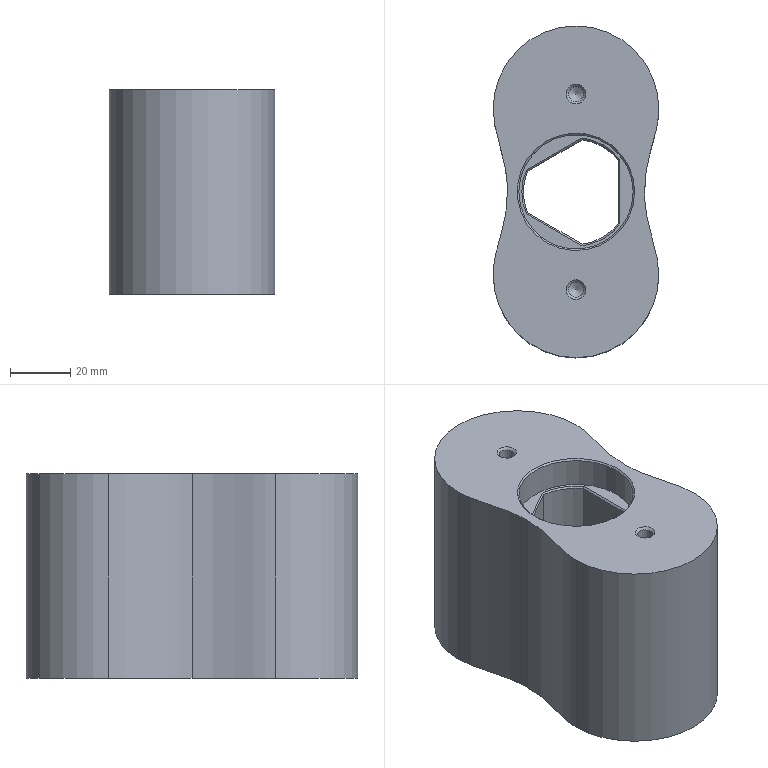NC program | NX | posted with a generic post | part box 55.004 x 110.159 x 68 mm
Lines 15415 to 16245 of 17802:
(CUTTERCOMP12 , TOOL : D12)
N30822 T12 M6
N30824 G54
N30826 G17 G0 G90 X-29.641 Y35.939 S5000 M3
N30828 G43 Z30. H12
N30830 Z1.
N30832 G94 G1 Z-1. F1250.
N30834 G41 X-29.607 Y35.845 D12
N30836 X-28.613 Y34.106
N30838 G3 X-27.576 Y33.502 R1.2
N30840 G2 X-20.525 Y32.77 R35.7
N30842 X-16.127 Y31.691 R60.387
N30844 G1 X-12.217 Y30.6
N30846 X-11.729 Y30.47
N30848 G3 X-6.353 Y29.294 R55.332
N30850 X6.353 Y29.294 R38.755
N30852 X11.729 Y30.47 R55.4
N30854 X16.345 Y31.754 R390.707
N30856 G2 X20.525 Y32.77 R61.951
N30858 X27.576 Y33.502 R35.718
N30860 X61.079 Y0.001 R33.502
N30862 X27.576 Y-33.502 R33.502
N30864 X20.525 Y-32.77 R35.7
N30866 X16.127 Y-31.691 R60.389
N30868 G1 X12.217 Y-30.6
N30870 X11.729 Y-30.47
N30872 G3 X6.353 Y-29.295 R55.338
N30874 X-6.353 Y-29.295 R38.754
N30876 X-11.729 Y-30.47 R55.381
N30878 X-16.345 Y-31.754 R390.608
N30880 G2 X-20.525 Y-32.77 R61.945
N30882 X-27.576 Y-33.502 R35.716
N30884 X-61.079 Y-0.001 R33.502
N30886 X-27.576 Y33.502 R33.502
N30888 G3 X-26.537 Y34.102 R1.2
N30890 G1 X-25.534 Y35.84
N30892 G40
N30894 X-25.5 Y35.934
N30896 Z1.
N30898 G0 X-29.641 Y35.939 Z0.
N30900 G1 Z-2.
N30902 G41 X-29.607 Y35.845
N30904 X-28.613 Y34.106
N30906 G3 X-27.576 Y33.502 R1.2
N30908 G2 X-20.525 Y32.77 R35.7
N30910 X-16.127 Y31.691 R60.387
N30912 G1 X-12.217 Y30.6
N30914 X-11.729 Y30.47
N30916 G3 X-6.353 Y29.295 R55.33
N30918 X6.353 Y29.295 R38.754
N30920 X11.729 Y30.47 R55.601
N30922 X16.345 Y31.754 R390.532
N30924 G2 X20.525 Y32.77 R61.937
N30926 X27.576 Y33.502 R35.715
N30928 X61.079 Y0.001 R33.502
N30930 X27.576 Y-33.502 R33.502
N30932 X20.036 Y-32.668 R36.091
N30934 X15.638 Y-31.556 R68.692
N30936 G3 X11.24 Y-30.342 R232.507
N30938 X5.864 Y-29.216 R53.118
N30940 X-6.353 Y-29.295 R38.762
N30942 X-11.729 Y-30.47 R55.563
N30944 X-16.345 Y-31.754 R390.333
N30946 G2 X-20.525 Y-32.77 R61.924
N30948 X-27.576 Y-33.502 R35.711
N30950 X-61.079 Y-0.001 R33.502
N30952 X-27.576 Y33.502 R33.502
N30954 G3 X-26.537 Y34.102 R1.2
N30956 G1 X-25.534 Y35.84
N30958 G40
N30960 X-25.5 Y35.934
N30962 Z0.
N30964 G0 X-29.641 Y35.939 Z-1.
N30966 G1 Z-3.
N30968 G41 X-29.607 Y35.845
N30970 X-28.613 Y34.106
N30972 G3 X-27.576 Y33.502 R1.2
N30974 G2 X-20.525 Y32.77 R35.7
N30976 X-16.127 Y31.691 R60.387
N30978 G1 X-12.217 Y30.6
N30980 X-11.729 Y30.47
N30982 G3 X-6.353 Y29.295 R55.328
N30984 X6.353 Y29.295 R38.753
N30986 X11.729 Y30.47 R55.578
N30988 X16.345 Y31.754 R390.357
N30990 G2 X20.525 Y32.77 R61.923
N30992 X27.576 Y33.502 R35.712
N30994 X61.079 Y0.001 R33.502
N30996 X27.576 Y-33.502 R33.502
N30998 X20.036 Y-32.669 R36.088
N31000 X15.638 Y-31.556 R68.743
N31002 G3 X11.24 Y-30.342 R232.194
N31004 X5.864 Y-29.216 R53.103
N31006 X-6.353 Y-29.295 R38.76
N31008 X-11.729 Y-30.47 R55.521
N31010 X-16.345 Y-31.754 R390.059
N31012 G2 X-20.525 Y-32.77 R61.903
N31014 X-27.576 Y-33.502 R35.706
N31016 X-61.079 Y-0.001 R33.502
N31018 X-27.576 Y33.502 R33.502
N31020 G3 X-26.537 Y34.102 R1.2
N31022 G1 X-25.534 Y35.84
N31024 G40
N31026 X-25.5 Y35.934
N31028 Z-1.
N31030 G0 X-29.641 Y35.939 Z-2.
N31032 G1 Z-4.
N31034 G41 X-29.607 Y35.845
N31036 X-28.613 Y34.106
N31038 G3 X-27.576 Y33.502 R1.2
N31040 G2 X-20.525 Y32.77 R35.7
N31042 X-16.127 Y31.691 R60.387
N31044 G1 X-12.217 Y30.6
N31046 X-11.729 Y30.47
N31048 G3 X-6.353 Y29.295 R55.326
N31050 X6.353 Y29.295 R38.752
N31052 X11.729 Y30.47 R55.555
N31054 X16.345 Y31.754 R390.181
N31056 G2 X20.525 Y32.77 R61.909
N31058 X27.576 Y33.502 R35.709
N31060 X61.079 Y0.001 R33.502
N31062 X27.576 Y-33.502 R33.502
N31064 X20.036 Y-32.669 R36.084
N31066 X15.638 Y-31.556 R68.794
N31068 G3 X11.24 Y-30.342 R231.881
N31070 X5.864 Y-29.216 R53.066
N31072 X-6.353 Y-29.295 R38.758
N31074 X-11.729 Y-30.47 R55.48
N31076 X-16.345 Y-31.754 R389.785
N31078 G2 X-20.525 Y-32.77 R61.882
N31080 X-27.576 Y-33.502 R35.629
N31082 X-61.079 Y-0.001 R33.502
N31084 X-27.576 Y33.502 R33.502
N31086 G3 X-26.537 Y34.102 R1.2
N31088 G1 X-25.534 Y35.84
N31090 G40
N31092 X-25.5 Y35.934
N31094 Z-2.
N31096 G0 X-29.638 Y35.939 Z-3.
N31098 G1 Z-5.
N31100 G41 X-29.605 Y35.845
N31102 X-28.612 Y34.107
N31104 G3 X-27.576 Y33.502 R1.2
N31106 G2 X-20.036 Y32.669 R36.084
N31108 X-15.638 Y31.556 R68.651
N31110 G3 X-11.24 Y30.342 R232.92
N31112 X-5.864 Y29.216 R53.116
N31114 X6.353 Y29.295 R38.761
N31116 X11.729 Y30.47 R55.532
N31118 X16.345 Y31.754 R390.007
N31120 G2 X20.525 Y32.77 R61.894
N31122 X27.576 Y33.502 R35.706
N31124 X61.079 Y0.001 R33.502
N31126 X27.576 Y-33.502 R33.502
N31128 X20.036 Y-32.669 R36.081
N31130 X15.638 Y-31.556 R68.83
N31132 G3 X11.24 Y-30.342 R231.57
N31134 X5.864 Y-29.217 R53.057
N31136 X-6.353 Y-29.295 R38.755
N31138 X-11.729 Y-30.47 R55.465
N31140 X-16.344 Y-31.754 R389.512
N31142 G2 X-20.525 Y-32.77 R61.861
N31144 X-27.576 Y-33.502 R35.624
N31146 X-61.079 Y-0.001 R33.502
N31148 X-27.576 Y33.502 R33.502
N31150 G3 X-26.537 Y34.102 R1.2
N31152 G1 X-25.534 Y35.839
N31154 G40
N31156 X-25.5 Y35.933
N31158 Z-3.
N31160 G0 X-29.641 Y35.939 Z-4.
N31162 G1 Z-6.
N31164 G41 X-29.607 Y35.845
N31166 X-28.613 Y34.106
N31168 G3 X-27.576 Y33.502 R1.2
N31170 G2 X-20.525 Y32.77 R35.701
N31172 X-16.127 Y31.691 R60.387
N31174 G1 X-12.217 Y30.6
N31176 X-11.729 Y30.47
N31178 G3 X-6.289 Y29.285 R54.809
N31180 X6.405 Y29.303 R38.597
N31182 X11.729 Y30.47 R55.51
N31184 X16.345 Y31.754 R389.832
N31186 G2 X20.525 Y32.77 R61.88
N31188 X27.576 Y33.502 R35.632
N31190 X61.079 Y0.001 R33.502
N31192 X27.576 Y-33.502 R33.502
N31194 X20.036 Y-32.669 R36.078
N31196 X15.638 Y-31.556 R68.857
N31198 G3 X11.24 Y-30.342 R231.258
N31200 X5.864 Y-29.217 R53.048
N31202 X-6.353 Y-29.295 R38.753
N31204 X-11.729 Y-30.47 R55.459
N31206 X-16.344 Y-31.754 R389.238
N31208 G2 X-20.525 Y-32.77 R61.84
N31210 X-27.576 Y-33.502 R35.619
N31212 X-61.079 Y-0.001 R33.502
N31214 X-27.576 Y33.502 R33.502
N31216 G3 X-26.537 Y34.102 R1.2
N31218 G1 X-25.534 Y35.84
N31220 G40
N31222 X-25.5 Y35.934
N31224 Z-4.
N31226 G0 X-29.641 Y35.939 Z-5.
N31228 G1 Z-7.
N31230 G41 X-29.607 Y35.845
N31232 X-28.613 Y34.106
N31234 G3 X-27.576 Y33.502 R1.2
N31236 G2 X-20.525 Y32.77 R35.7
N31238 X-16.127 Y31.691 R60.387
N31240 G1 X-12.217 Y30.6
N31242 X-11.729 Y30.47
N31244 G3 X-6.287 Y29.284 R54.784
N31246 X6.402 Y29.303 R38.597
N31248 X11.729 Y30.47 R55.487
N31250 X16.345 Y31.754 R389.657
N31252 G2 X20.525 Y32.77 R61.866
N31254 X27.576 Y33.502 R35.629
N31256 X61.079 Y0.001 R33.502
N31258 X27.576 Y-33.502 R33.502
N31260 X20.036 Y-32.669 R36.074
N31262 X15.638 Y-31.556 R68.884
N31264 G3 X11.24 Y-30.342 R233.491
N31266 X5.864 Y-29.217 R53.039
N31268 X-6.353 Y-29.295 R38.751
N31270 X-11.729 Y-30.47 R55.356
N31272 X-16.344 Y-31.754 R388.965
N31274 G2 X-20.525 Y-32.77 R61.819
N31276 X-27.576 Y-33.502 R35.613
N31278 X-61.079 Y-0.001 R33.502
N31280 X-27.576 Y33.502 R33.502
N31282 G3 X-26.537 Y34.102 R1.2
N31284 G1 X-25.534 Y35.84
N31286 G40
N31288 X-25.5 Y35.934
N31290 Z-5.
N31292 G0 X-29.641 Y35.939 Z-6.
N31294 G1 Z-8.
N31296 G41 X-29.607 Y35.845
N31298 X-28.613 Y34.106
N31300 G3 X-27.576 Y33.502 R1.2
N31302 G2 X-20.525 Y32.77 R35.697
N31304 X-16.127 Y31.692 R60.387
N31306 G1 X-12.217 Y30.6
N31308 X-11.729 Y30.47
N31310 G3 X-6.284 Y29.284 R54.759
N31312 X6.401 Y29.303 R38.597
N31314 X11.729 Y30.47 R55.477
N31316 X16.345 Y31.754 R389.483
N31318 G2 X20.525 Y32.77 R61.852
N31320 X27.576 Y33.502 R35.626
N31322 X61.079 Y0.001 R33.502
N31324 X27.576 Y-33.502 R33.502
N31326 X20.036 Y-32.669 R36.071
N31328 X15.638 Y-31.556 R68.911
N31330 G3 X11.24 Y-30.342 R232.675
N31332 X5.864 Y-29.217 R53.028
N31334 X-6.353 Y-29.295 R38.749
N31336 X-11.729 Y-30.47 R55.538
N31338 X-16.344 Y-31.754 R388.692
N31340 G2 X-20.525 Y-32.77 R61.798
N31342 X-27.576 Y-33.502 R35.679
N31344 X-61.079 Y-0.001 R33.502
N31346 X-27.576 Y33.502 R33.502
N31348 G3 X-26.537 Y34.102 R1.2
N31350 G1 X-25.534 Y35.84
N31352 G40
N31354 X-25.499 Y35.934
N31356 Z-6.
N31358 G0 X-29.641 Y35.939 Z-7.
N31360 G1 Z-9.
N31362 G41 X-29.607 Y35.845
N31364 X-28.613 Y34.106
N31366 G3 X-27.576 Y33.502 R1.2
N31368 G2 X-20.525 Y32.77 R35.694
N31370 X-16.127 Y31.692 R60.387
N31372 G1 X-12.217 Y30.6
N31374 X-11.729 Y30.47
N31376 G3 X-6.281 Y29.284 R54.734
N31378 X6.401 Y29.303 R38.597
N31380 X11.729 Y30.47 R55.475
N31382 X16.345 Y31.754 R389.308
N31384 G2 X20.525 Y32.77 R61.837
N31386 X27.576 Y33.502 R35.623
N31388 X61.079 Y0.001 R33.502
N31390 X27.576 Y-33.502 R33.502
N31392 X20.036 Y-32.669 R36.068
N31394 X15.638 Y-31.556 R68.938
N31396 G3 X11.24 Y-30.343 R231.865
N31398 X5.864 Y-29.217 R53.013
N31400 X-6.353 Y-29.295 R38.747
N31402 X-11.729 Y-30.47 R55.383
N31404 X-16.344 Y-31.754 R388.42
N31406 G2 X-20.525 Y-32.77 R61.777
N31408 X-27.576 Y-33.502 R35.674
N31410 X-61.079 Y-0.001 R33.502
N31412 X-27.576 Y33.502 R33.502
N31414 G3 X-26.537 Y34.102 R1.2
N31416 G1 X-25.534 Y35.84
N31418 G40
N31420 X-25.499 Y35.934
N31422 Z-7.
N31424 G0 X-29.64 Y35.939 Z-8.
N31426 G1 Z-10.
N31428 G41 X-29.607 Y35.845
N31430 X-28.613 Y34.107
N31432 G3 X-27.576 Y33.502 R1.2
N31434 G2 X-20.525 Y32.77 R35.762
N31436 X-16.127 Y31.692 R60.387
N31438 G1 X-12.217 Y30.6
N31440 X-11.729 Y30.47
N31442 G3 X-6.279 Y29.283 R54.709
N31444 X6.401 Y29.303 R38.597
N31446 X11.729 Y30.47 R55.473
N31448 X16.344 Y31.754 R389.134
N31450 G2 X20.525 Y32.77 R61.823
N31452 X27.576 Y33.502 R35.62
N31454 X61.079 Y0.001 R33.502
N31456 X27.576 Y-33.502 R33.502
N31458 X20.036 Y-32.669 R36.064
N31460 X15.638 Y-31.556 R68.966
N31462 G3 X11.24 Y-30.343 R231.061
N31464 X5.864 Y-29.217 R52.998
N31466 X-6.353 Y-29.295 R38.745
N31468 X-11.729 Y-30.47 R55.353
N31470 X-16.127 Y-31.694 R357.038
N31472 G2 X-20.525 Y-32.77 R62.337
N31474 X-27.576 Y-33.502 R35.669
N31476 X-61.079 Y-0.001 R33.502
N31478 X-27.576 Y33.502 R33.502
N31480 G3 X-26.537 Y34.102 R1.2
N31482 G1 X-25.534 Y35.839
N31484 G40
N31486 X-25.5 Y35.933
N31488 Z-8.
N31490 G0 X-29.64 Y35.939 Z-9.
N31492 G1 Z-11.
N31494 G41 X-29.607 Y35.845
N31496 X-28.613 Y34.107
N31498 G3 X-27.576 Y33.502 R1.2
N31500 G2 X-20.525 Y32.77 R35.759
N31502 X-16.127 Y31.692 R60.387
N31504 G1 X-12.217 Y30.6
N31506 X-11.729 Y30.47
N31508 G3 X-6.276 Y29.283 R54.684
N31510 X6.4 Y29.303 R38.597
N31512 X11.729 Y30.47 R55.471
N31514 X16.344 Y31.754 R388.96
N31516 G2 X20.525 Y32.77 R61.809
N31518 X27.576 Y33.502 R35.617
N31520 X61.079 Y0.001 R33.502
N31522 X27.576 Y-33.502 R33.502
N31524 X20.036 Y-32.669 R36.061
N31526 X15.638 Y-31.556 R68.993
N31528 G3 X11.24 Y-30.343 R230.262
N31530 X5.864 Y-29.217 R52.983
N31532 X-6.353 Y-29.295 R38.743
N31534 X-11.729 Y-30.47 R55.43
N31536 X-16.127 Y-31.694 R356.256
N31538 G2 X-20.525 Y-32.77 R62.337
N31540 X-27.576 Y-33.502 R35.664
N31542 X-61.079 Y-0.001 R33.502
N31544 X-27.576 Y33.502 R33.502
N31546 G3 X-26.537 Y34.102 R1.2
N31548 G1 X-25.534 Y35.839
N31550 G40
N31552 X-25.5 Y35.933
N31554 Z-9.
N31556 G0 X-29.641 Y35.939 Z-10.
N31558 G1 Z-12.
N31560 G41 X-29.607 Y35.845
N31562 X-28.613 Y34.107
N31564 G3 X-27.576 Y33.502 R1.2
N31566 G2 X-20.525 Y32.77 R35.756
N31568 X-16.127 Y31.692 R60.387
N31570 G1 X-12.217 Y30.6
N31572 X-11.729 Y30.47
N31574 G3 X-5.864 Y29.217 R54.659
N31576 X6.353 Y29.295 R38.753
N31578 X11.729 Y30.47 R55.374
N31580 X16.344 Y31.754 R388.786
N31582 G2 X20.525 Y32.77 R61.795
N31584 X27.576 Y33.502 R35.614
N31586 X61.079 Y0.001 R33.502
N31588 X27.576 Y-33.502 R33.502
N31590 X20.036 Y-32.669 R36.057
N31592 X15.638 Y-31.556 R69.02
N31594 G3 X11.24 Y-30.343 R229.468
N31596 X5.864 Y-29.217 R52.968
N31598 X-6.353 Y-29.295 R38.74
N31600 X-11.729 Y-30.471 R55.424
N31602 X-16.127 Y-31.694 R355.478
N31604 G2 X-20.525 Y-32.77 R62.337
N31606 X-27.576 Y-33.502 R35.658
N31608 X-61.079 Y-0.001 R33.502
N31610 X-27.576 Y33.502 R33.502
N31612 G3 X-26.537 Y34.102 R1.2
N31614 G1 X-25.534 Y35.839
N31616 G40
N31618 X-25.5 Y35.933
N31620 Z-10.
N31622 G0 X-29.641 Y35.939 Z-11.
N31624 G1 Z-13.
N31626 G41 X-29.607 Y35.845
N31628 X-28.613 Y34.107
N31630 G3 X-27.576 Y33.502 R1.2
N31632 G2 X-20.525 Y32.77 R35.753
N31634 X-16.127 Y31.692 R60.387
N31636 G1 X-12.217 Y30.6
N31638 X-11.729 Y30.47
N31640 G3 X-5.864 Y29.217 R54.657
N31642 X6.353 Y29.295 R38.752
N31644 X11.729 Y30.47 R55.575
N31646 X16.344 Y31.754 R388.613
N31648 G2 X20.525 Y32.77 R61.781
N31650 X27.576 Y33.502 R35.611
N31652 X61.079 Y0.001 R33.502
N31654 X27.576 Y-33.502 R33.502
N31656 X20.036 Y-32.669 R36.054
N31658 X15.638 Y-31.557 R69.536
N31660 G3 X11.24 Y-30.343 R228.68
N31662 X5.864 Y-29.217 R52.953
N31664 X-6.353 Y-29.295 R38.738
N31666 X-11.729 Y-30.471 R55.418
N31668 X-16.127 Y-31.694 R354.703
N31670 G2 X-20.525 Y-32.77 R62.338
N31672 X-27.576 Y-33.502 R35.653
N31674 X-61.079 Y-0.001 R33.502
N31676 X-27.576 Y33.502 R33.502
N31678 G3 X-26.537 Y34.102 R1.2
N31680 G1 X-25.534 Y35.839
N31682 G40
N31684 X-25.5 Y35.933
N31686 Z-11.
N31688 G0 X-29.641 Y35.939 Z-12.
N31690 G1 Z-14.
N31692 G41 X-29.607 Y35.845
N31694 X-28.613 Y34.107
N31696 G3 X-27.576 Y33.502 R1.2
N31698 G2 X-20.525 Y32.77 R35.75
N31700 X-16.127 Y31.692 R60.387
N31702 G1 X-12.217 Y30.6
N31704 X-11.729 Y30.47
N31706 G3 X-5.864 Y29.217 R54.656
N31708 X6.353 Y29.295 R38.751
N31710 X11.729 Y30.47 R55.552
N31712 X16.344 Y31.754 R388.439
N31714 G2 X20.525 Y32.77 R61.783
N31716 X27.576 Y33.502 R35.608
N31718 X61.079 Y0.001 R33.502
N31720 X27.576 Y-33.502 R33.502
N31722 X20.036 Y-32.669 R36.051
N31724 X15.638 Y-31.557 R69.562
N31726 G3 X11.24 Y-30.343 R227.898
N31728 X5.864 Y-29.217 R52.939
N31730 X-6.353 Y-29.295 R38.736
N31732 X-11.729 Y-30.471 R55.413
N31734 X-16.127 Y-31.694 R353.931
N31736 G2 X-20.525 Y-32.77 R62.338
N31738 X-27.576 Y-33.502 R35.648
N31740 X-61.079 Y-0.001 R33.502
N31742 X-27.576 Y33.502 R33.502
N31744 G3 X-26.537 Y34.102 R1.2
N31746 G1 X-25.534 Y35.839
N31748 G40
N31750 X-25.5 Y35.933
N31752 Z-12.
N31754 G0 X-29.641 Y35.939 Z-13.
N31756 G1 Z-15.
N31758 G41 X-29.607 Y35.845
N31760 X-28.613 Y34.106
N31762 G3 X-27.576 Y33.502 R1.2
N31764 G2 X-20.525 Y32.77 R35.747
N31766 X-16.127 Y31.692 R60.387
N31768 G1 X-12.217 Y30.6
N31770 X-11.729 Y30.47
N31772 G3 X-5.864 Y29.217 R54.654
N31774 X6.353 Y29.295 R38.75
N31776 X11.729 Y30.47 R55.529
N31778 X16.344 Y31.754 R388.266
N31780 G2 X20.525 Y32.77 R61.769
N31782 X27.576 Y33.502 R35.605
N31784 X61.079 Y0.001 R33.502
N31786 X27.576 Y-33.502 R33.502
N31788 X20.036 Y-32.669 R36.047
N31790 X15.638 Y-31.557 R69.588
N31792 G3 X11.24 Y-30.343 R227.121
N31794 X5.864 Y-29.217 R52.924
N31796 X-6.353 Y-29.295 R38.734
N31798 X-11.729 Y-30.471 R55.407
N31800 X-16.127 Y-31.694 R353.163
N31802 G2 X-20.525 Y-32.77 R62.274
N31804 X-27.576 Y-33.502 R35.643
N31806 X-61.079 Y-0.001 R33.502
N31808 X-27.576 Y33.502 R33.502
N31810 G3 X-26.537 Y34.102 R1.2
N31812 G1 X-25.534 Y35.839
N31814 G40
N31816 X-25.5 Y35.933
N31818 Z-13.
N31820 G0 X-29.641 Y35.939 Z-14.
N31822 G1 Z-16.
N31824 G41 X-29.607 Y35.845
N31826 X-28.613 Y34.106
N31828 G3 X-27.576 Y33.502 R1.2
N31830 G2 X-20.525 Y32.77 R35.744
N31832 X-16.127 Y31.692 R60.387
N31834 G1 X-12.217 Y30.6
N31836 X-11.729 Y30.47
N31838 G3 X-5.864 Y29.217 R54.652
N31840 X6.353 Y29.295 R38.749
N31842 X11.729 Y30.47 R55.397
N31844 X16.344 Y31.754 R388.092
N31846 G2 X20.525 Y32.77 R61.755
N31848 X27.576 Y33.502 R35.602
N31850 X61.079 Y0.001 R33.502
N31852 X27.576 Y-33.502 R33.502
N31854 X20.036 Y-32.669 R36.044
N31856 X15.638 Y-31.557 R69.614
N31858 G3 X11.24 Y-30.343 R226.349
N31860 X5.864 Y-29.217 R52.909
N31862 X-6.353 Y-29.295 R38.732
N31864 X-11.729 Y-30.471 R55.392
N31866 X-16.344 Y-31.754 R399.417
N31868 G2 X-20.525 Y-32.77 R61.58
N31870 X-27.576 Y-33.502 R35.637
N31872 X-61.079 Y-0.001 R33.502
N31874 X-27.576 Y33.502 R33.502
N31876 G3 X-26.537 Y34.102 R1.2
N31878 G1 X-25.534 Y35.84
N31880 G40
N31882 X-25.5 Y35.933
N31884 Z-14.
N31886 G0 X-29.641 Y35.939 Z-15.
N31888 G1 Z-17.
N31890 G41 X-29.607 Y35.845
N31892 X-28.613 Y34.106
N31894 G3 X-27.576 Y33.502 R1.2
N31896 G2 X-20.525 Y32.77 R35.741
N31898 X-16.127 Y31.692 R60.387
N31900 G1 X-12.217 Y30.6
N31902 X-11.729 Y30.47
N31904 G3 X-5.864 Y29.217 R54.651
N31906 X6.353 Y29.295 R38.748
N31908 X11.729 Y30.47 R55.38
N31910 X16.127 Y31.694 R353.605
N31912 G2 X20.525 Y32.77 R62.411
N31914 X27.576 Y33.502 R35.599
N31916 X61.079 Y0.001 R33.502
N31918 X27.576 Y-33.502 R33.502
N31920 X20.036 Y-32.669 R36.041
N31922 X15.638 Y-31.557 R69.64
N31924 G3 X11.24 Y-30.343 R230.134
N31926 X5.864 Y-29.217 R52.894
N31928 X-6.842 Y-29.376 R39.076
N31930 X-12.706 Y-30.734 R62.719
N31932 G1 X-13.195 Y-30.87
N31934 X-16.344 Y-31.754
N31936 X-17.104 Y-31.959
N31938 G2 X-21.933 Y-33.028 R49.242
N31940 X-27.074 Y-33.498 R33.876
N31942 X-27.576 Y33.502 R-33.502
N31944 G3 X-26.537 Y34.102 R1.2
N31946 G1 X-25.534 Y35.84
N31948 G40
N31950 X-25.5 Y35.933
N31952 Z-15.
N31954 G0 X-29.641 Y35.939 Z-16.
N31956 G1 Z-18.
N31958 G41 X-29.607 Y35.845
N31960 X-28.613 Y34.106
N31962 G3 X-27.576 Y33.502 R1.2
N31964 G2 X-20.525 Y32.77 R35.738
N31966 X-16.127 Y31.692 R60.387
N31968 G1 X-12.217 Y30.6
N31970 X-11.729 Y30.47
N31972 G3 X-5.864 Y29.217 R54.649
N31974 X6.353 Y29.295 R38.746
N31976 X11.729 Y30.47 R55.364
N31978 X16.127 Y31.694 R352.954
N31980 G2 X20.525 Y32.77 R62.416
N31982 X27.576 Y33.502 R35.596
N31984 X61.079 Y0.001 R33.502
N31986 X27.576 Y-33.502 R33.502
N31988 X20.036 Y-32.669 R36.037
N31990 X15.638 Y-31.557 R69.665
N31992 G3 X11.24 Y-30.343 R229.341
N31994 X5.864 Y-29.217 R52.879
N31996 X-6.842 Y-29.376 R39.047
N31998 X-12.706 Y-30.734 R62.705
N32000 G1 X-13.195 Y-30.87
N32002 X-16.344 Y-31.754
N32004 X-17.104 Y-31.959
N32006 G2 X-21.929 Y-33.027 R49.264
N32008 X-27.076 Y-33.498 R33.879
N32010 X-27.576 Y33.502 R-33.502
N32012 G3 X-26.537 Y34.102 R1.2
N32014 G1 X-25.534 Y35.84
N32016 G40
N32018 X-25.5 Y35.934
N32020 Z-16.
N32022 G0 X-29.641 Y35.939 Z-17.
N32024 G1 Z-19.
N32026 G41 X-29.607 Y35.845
N32028 X-28.613 Y34.106
N32030 G3 X-27.576 Y33.502 R1.2
N32032 G2 X-20.525 Y32.77 R35.735
N32034 X-16.127 Y31.692 R60.387
N32036 G1 X-12.217 Y30.6
N32038 X-11.729 Y30.47
N32040 G3 X-5.864 Y29.217 R54.648
N32042 X6.353 Y29.295 R38.745
N32044 X11.729 Y30.47 R55.455
N32046 X16.127 Y31.694 R352.306
N32048 G2 X20.525 Y32.77 R62.421
N32050 X27.576 Y33.502 R35.593
N32052 X61.079 Y0.001 R33.502
N32054 X27.576 Y-33.502 R33.502
N32056 X20.036 Y-32.669 R36.034
N32058 X15.638 Y-31.557 R69.691
N32060 G3 X11.24 Y-30.343 R228.555
N32062 X5.864 Y-29.217 R52.864
N32064 X-6.842 Y-29.376 R39.017
N32066 X-12.706 Y-30.734 R62.692
N32068 G1 X-13.195 Y-30.87
N32070 X-16.344 Y-31.754
N32072 X-17.104 Y-31.959
N32074 G2 X-21.924 Y-33.026 R49.286
N32076 X-27.079 Y-33.498 R33.883
N32078 X-27.576 Y33.502 R-33.502
N32080 G3 X-26.537 Y34.102 R1.2
N32082 G1 X-25.534 Y35.84
N32084 G40
N32086 X-25.5 Y35.934
N32088 Z-17.
N32090 G0 X-29.641 Y35.939 Z-18.
N32092 G1 Z-20.
N32094 G41 X-29.607 Y35.845
N32096 X-28.613 Y34.106
N32098 G3 X-27.576 Y33.502 R1.2
N32100 G2 X-20.525 Y32.77 R35.732
N32102 X-16.127 Y31.692 R60.387
N32104 G1 X-12.217 Y30.6
N32106 X-11.729 Y30.471
N32108 G3 X-5.864 Y29.217 R54.646
N32110 X6.353 Y29.295 R38.744
N32112 X11.729 Y30.471 R55.453
N32114 X16.127 Y31.694 R351.66
N32116 G2 X20.525 Y32.77 R62.425
N32118 X27.576 Y33.502 R35.59
N32120 X61.079 Y0.001 R33.502
N32122 X27.576 Y-33.502 R33.502
N32124 X20.036 Y-32.669 R36.031
N32126 X15.638 Y-31.557 R69.717
N32128 G3 X11.24 Y-30.343 R227.773
N32130 X5.864 Y-29.217 R52.849
N32132 X-6.842 Y-29.376 R38.987
N32134 X-12.706 Y-30.734 R62.678
N32136 G1 X-13.195 Y-30.87
N32138 X-16.344 Y-31.754
N32140 X-17.104 Y-31.959
N32142 G2 X-21.919 Y-33.026 R49.308
N32144 X-27.081 Y-33.498 R33.887
N32146 X-27.576 Y33.502 R-33.502
N32148 G3 X-26.537 Y34.102 R1.2
N32150 G1 X-25.534 Y35.84
N32152 G40
N32154 X-25.5 Y35.934
N32156 Z-18.
N32158 G0 X-29.641 Y35.939 Z-19.
N32160 G1 Z-21.
N32162 G41 X-29.607 Y35.845
N32164 X-28.613 Y34.106
N32166 G3 X-27.576 Y33.502 R1.2
N32168 G2 X-20.525 Y32.77 R35.729
N32170 X-16.127 Y31.692 R60.387
N32172 G1 X-12.217 Y30.6
N32174 X-11.729 Y30.471
N32176 G3 X-5.864 Y29.217 R54.644
N32178 X6.353 Y29.295 R38.743
N32180 X11.729 Y30.471 R55.451
N32182 X16.127 Y31.694 R351.016
N32184 G2 X20.525 Y32.77 R62.43
N32186 X27.576 Y33.502 R35.587
N32188 X61.079 Y0.001 R33.502
N32190 X27.576 Y-33.502 R33.502
N32192 X20.036 Y-32.669 R36.027
N32194 X15.638 Y-31.557 R69.743
N32196 G3 X11.24 Y-30.343 R226.997
N32198 X5.864 Y-29.217 R52.834
N32200 X-6.353 Y-29.295 R38.721
N32202 X-12.217 Y-30.601 R58.289
N32204 G1 X-12.706 Y-30.734
N32206 X-16.344 Y-31.754
N32208 X-17.104 Y-31.959
N32210 G2 X-21.915 Y-33.025 R49.33
N32212 X-27.084 Y-33.499 R33.891
N32214 X-27.576 Y33.502 R-33.502
N32216 G3 X-26.537 Y34.102 R1.2
N32218 G1 X-25.534 Y35.84
N32220 G40
N32222 X-25.5 Y35.934
N32224 Z-19.
N32226 G0 X-29.641 Y35.939 Z-20.
N32228 G1 Z-22.
N32230 G41 X-29.607 Y35.845
N32232 X-28.613 Y34.106
N32234 G3 X-27.576 Y33.502 R1.2
N32236 G2 X-20.525 Y32.77 R35.726
N32238 X-16.127 Y31.692 R60.387
N32240 G1 X-12.217 Y30.6
N32242 X-11.729 Y30.471
N32244 G3 X-5.864 Y29.217 R54.643
N32246 X6.353 Y29.295 R38.742
N32248 X11.729 Y30.471 R55.449
N32250 X16.127 Y31.694 R350.375
N32252 G2 X20.525 Y32.77 R62.434
N32254 X27.576 Y33.502 R35.584
N32256 X61.079 Y0.001 R33.502
N32258 X27.576 Y-33.502 R33.502
N32260 X20.525 Y-32.77 R35.627
N32262 X16.127 Y-31.692 R61.188
N32264 G1 X12.217 Y-30.601
N32266 X11.729 Y-30.471
N32268 G3 X5.864 Y-29.217 R54.454
N32270 X-6.353 Y-29.295 R38.719
N32272 X-12.217 Y-30.601 R58.247
N32274 G1 X-16.344 Y-31.754
N32276 X-17.104 Y-31.959
N32278 G2 X-21.91 Y-33.024 R49.352
N32280 X-27.086 Y-33.499 R33.895
N32282 X-27.576 Y33.502 R-33.502
N32284 G3 X-26.537 Y34.102 R1.2
N32286 G1 X-25.534 Y35.84
N32288 G40
N32290 X-25.5 Y35.934
N32292 Z-20.
N32294 G0 X-29.641 Y35.939 Z-21.
N32296 G1 Z-23.
N32298 G41 X-29.607 Y35.845
N32300 X-28.613 Y34.106
N32302 G3 X-27.576 Y33.502 R1.2
N32304 G2 X-20.525 Y32.77 R35.723
N32306 X-16.127 Y31.692 R60.387
N32308 G1 X-12.217 Y30.6
N32310 X-11.729 Y30.471
N32312 G3 X-5.864 Y29.217 R54.641
N32314 X6.353 Y29.295 R38.741
N32316 X11.729 Y30.471 R55.447
N32318 X16.127 Y31.694 R349.736
N32320 G2 X20.525 Y32.77 R62.439
N32322 X27.576 Y33.502 R35.581
N32324 X61.079 Y0.001 R33.502
N32326 X27.576 Y-33.502 R33.502
N32328 X20.525 Y-32.77 R35.623
N32330 X16.127 Y-31.692 R61.2
N32332 G1 X12.217 Y-30.601
N32334 X11.729 Y-30.471
N32336 G3 X5.864 Y-29.217 R54.422
N32338 X-6.353 Y-29.295 R38.717
N32340 X-12.217 Y-30.601 R58.204
N32342 G1 X-16.344 Y-31.754
N32344 X-17.104 Y-31.959
N32346 G2 X-21.906 Y-33.023 R49.374
N32348 X-27.089 Y-33.499 R33.899
N32350 X-27.576 Y33.502 R-33.502
N32352 G3 X-26.537 Y34.102 R1.2
N32354 G1 X-25.534 Y35.84
N32356 G40
N32358 X-25.499 Y35.934
N32360 Z-21.
N32362 G0 X-29.641 Y35.939 Z-22.
N32364 G1 Z-24.
N32366 G41 X-29.607 Y35.845
N32368 X-28.613 Y34.106
N32370 G3 X-27.576 Y33.502 R1.2
N32372 G2 X-20.525 Y32.77 R35.72
N32374 X-16.127 Y31.692 R60.387
N32376 G1 X-12.217 Y30.6
N32378 X-11.729 Y30.471
N32380 G3 X-5.864 Y29.217 R54.64
N32382 X6.353 Y29.295 R38.74
N32384 X11.729 Y30.471 R55.445
N32386 X16.127 Y31.694 R349.099
N32388 G2 X20.525 Y32.77 R62.444
N32390 X27.576 Y33.502 R35.578
N32392 X61.079 Y0.001 R33.502
N32394 X27.576 Y-33.502 R33.502
N32396 X20.525 Y-32.771 R35.618
N32398 X16.127 Y-31.692 R61.213
N32400 G1 X12.217 Y-30.601
N32402 X11.729 Y-30.471
N32404 G3 X5.864 Y-29.218 R54.389
N32406 X-6.353 Y-29.295 R38.715
N32408 X-12.217 Y-30.601 R58.162
N32410 G1 X-16.344 Y-31.754
N32412 X-17.104 Y-31.959
N32414 G2 X-21.901 Y-33.023 R49.397
N32416 X-27.091 Y-33.499 R33.902
N32418 X-27.576 Y33.502 R-33.502
N32420 G3 X-26.537 Y34.102 R1.2
N32422 G1 X-25.534 Y35.84
N32424 G40
N32426 X-25.499 Y35.934
N32428 Z-22.
N32430 G0 X-29.641 Y35.939 Z-23.
N32432 G1 Z-25.
N32434 G41 X-29.607 Y35.845
N32436 X-28.613 Y34.106
N32438 G3 X-27.576 Y33.502 R1.2
N32440 G2 X-20.525 Y32.77 R35.717
N32442 X-16.127 Y31.692 R60.387
N32444 G1 X-12.217 Y30.6
N32446 X-11.729 Y30.471
N32448 G3 X-5.864 Y29.217 R54.638
N32450 X6.353 Y29.295 R38.739
N32452 X11.729 Y30.471 R55.443
N32454 X16.127 Y31.694 R348.465
N32456 G2 X20.525 Y32.77 R62.448
N32458 X27.576 Y33.502 R35.575
N32460 X61.079 Y0.001 R33.502
N32462 X27.576 Y-33.502 R33.502
N32464 X20.525 Y-32.771 R35.614
N32466 X16.127 Y-31.693 R61.225
N32468 G1 X12.217 Y-30.601
N32470 X11.729 Y-30.471
N32472 G3 X5.864 Y-29.218 R54.749
N32474 X-6.353 Y-29.296 R38.712
N32476 X-12.217 Y-30.601 R58.12